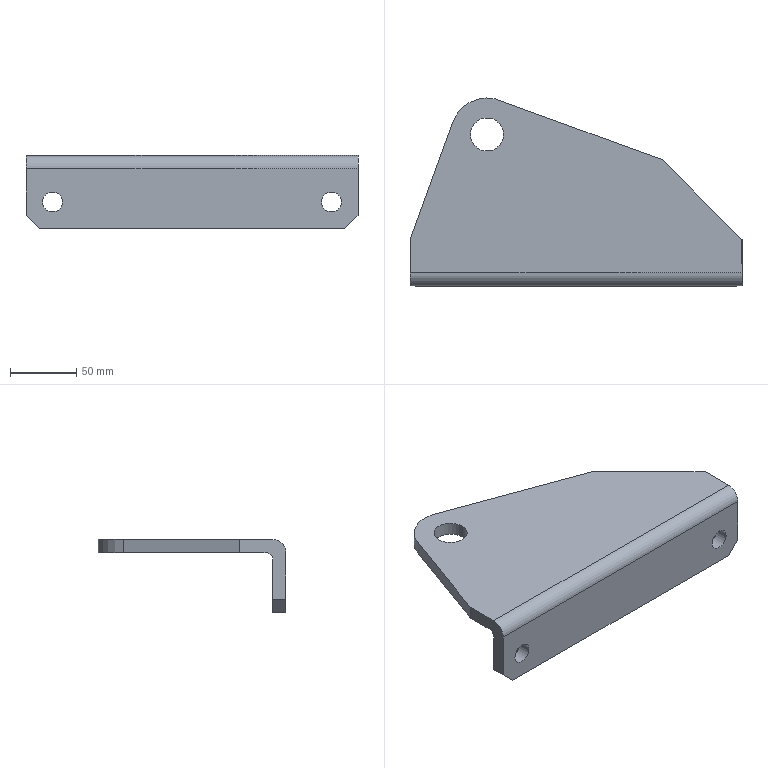Part | SolidWorks | features ICE 4, Fillet 2, Chamfer 1, Extrusion 1 | 1 solid | 21 faces | box 250 x 141.5 x 55 mm | volume 355868 mm3 | plane 12 | cylinder 9 | commonest cylinder face diameters 15 x4 25 x2 10 x1 20 x1 55 x1
STEP:
#1=CARTESIAN_POINT('',(-112.5,-80.5,-25.));
#2=VERTEX_POINT('',#1);
#3=CARTESIAN_POINT('',(-97.5,-80.5,-25.));
#4=VERTEX_POINT('',#3);
#5=CARTESIAN_POINT('',(-105.,-80.5,-25.));
#6=DIRECTION('',(0.,-1.,0.));
#7=DIRECTION('',(0.,0.,-1.));
#8=AXIS2_PLACEMENT_3D('',#5,#6,#7);
#9=CIRCLE('',#8,7.5);
#10=EDGE_CURVE('',#2,#4,#9,.T.);
#11=ORIENTED_EDGE('',*,*,#10,.F.);
#12=CARTESIAN_POINT('',(-112.5,-90.5,-25.));
#13=VERTEX_POINT('',#12);
#14=CARTESIAN_POINT('',(-112.5,-45.5,-25.));
#15=DIRECTION('',(0.,-1.,0.));
#16=VECTOR('',#15,1000.);
#17=LINE('',#14,#16);
#18=EDGE_CURVE('',#2,#13,#17,.T.);
#19=ORIENTED_EDGE('',*,*,#18,.T.);
#20=CARTESIAN_POINT('',(-97.5,-90.5,-25.));
#21=VERTEX_POINT('',#20);
#22=CARTESIAN_POINT('',(-105.,-90.5,-25.));
#23=DIRECTION('',(0.,-1.,0.));
#24=DIRECTION('',(1.,0.,0.));
#25=AXIS2_PLACEMENT_3D('',#22,#23,#24);
#26=CIRCLE('',#25,7.5);
#27=EDGE_CURVE('',#13,#21,#26,.T.);
#28=ORIENTED_EDGE('',*,*,#27,.T.);
#29=CARTESIAN_POINT('',(-97.5,-45.5,-25.));
#30=DIRECTION('',(0.,-1.,0.));
#31=VECTOR('',#30,1000.);
#32=LINE('',#29,#31);
#33=EDGE_CURVE('',#4,#21,#32,.T.);
#34=ORIENTED_EDGE('',*,*,#33,.F.);
#35=EDGE_LOOP('',(#11,#19,#28,#34));
#36=FACE_OUTER_BOUND('',#35,.T.);
#37=CARTESIAN_POINT('',(-105.,-45.5,-25.));
#38=DIRECTION('',(0.,-1.,0.));
#39=DIRECTION('',(1.,0.,0.));
#40=AXIS2_PLACEMENT_3D('',#37,#38,#39);
#41=CYLINDRICAL_SURFACE('',#40,7.5);
#42=ADVANCED_FACE('',(#36),#41,.F.);
#43=CARTESIAN_POINT('',(97.5,-80.5,-25.));
#44=VERTEX_POINT('',#43);
#45=CARTESIAN_POINT('',(112.5,-80.5,-25.));
#46=VERTEX_POINT('',#45);
#47=CARTESIAN_POINT('',(105.,-80.5,-25.));
#48=DIRECTION('',(0.,-1.,0.));
#49=DIRECTION('',(0.,0.,-1.));
#50=AXIS2_PLACEMENT_3D('',#47,#48,#49);
#51=CIRCLE('',#50,7.5);
#52=EDGE_CURVE('',#44,#46,#51,.T.);
#53=ORIENTED_EDGE('',*,*,#52,.F.);
#54=CARTESIAN_POINT('',(97.5,-90.5,-25.));
#55=VERTEX_POINT('',#54);
#56=CARTESIAN_POINT('',(97.5,-45.5,-25.));
#57=DIRECTION('',(0.,-1.,0.));
#58=VECTOR('',#57,1000.);
#59=LINE('',#56,#58);
#60=EDGE_CURVE('',#44,#55,#59,.T.);
#61=ORIENTED_EDGE('',*,*,#60,.T.);
#62=CARTESIAN_POINT('',(112.5,-90.5,-25.));
#63=VERTEX_POINT('',#62);
#64=CARTESIAN_POINT('',(105.,-90.5,-25.));
#65=DIRECTION('',(0.,-1.,0.));
#66=DIRECTION('',(1.,0.,0.));
#67=AXIS2_PLACEMENT_3D('',#64,#65,#66);
#68=CIRCLE('',#67,7.5);
#69=EDGE_CURVE('',#55,#63,#68,.T.);
#70=ORIENTED_EDGE('',*,*,#69,.T.);
#71=CARTESIAN_POINT('',(112.5,-45.5,-25.));
#72=DIRECTION('',(0.,-1.,0.));
#73=VECTOR('',#72,1000.);
#74=LINE('',#71,#73);
#75=EDGE_CURVE('',#46,#63,#74,.T.);
#76=ORIENTED_EDGE('',*,*,#75,.F.);
#77=EDGE_LOOP('',(#53,#61,#70,#76));
#78=FACE_OUTER_BOUND('',#77,.T.);
#79=CARTESIAN_POINT('',(105.,-45.5,-25.));
#80=DIRECTION('',(0.,-1.,0.));
#81=DIRECTION('',(1.,0.,0.));
#82=AXIS2_PLACEMENT_3D('',#79,#80,#81);
#83=CYLINDRICAL_SURFACE('',#82,7.5);
#84=ADVANCED_FACE('',(#78),#83,.F.);
#85=CARTESIAN_POINT('',(-79.5,23.5,0.));
#86=VERTEX_POINT('',#85);
#87=CARTESIAN_POINT('',(-54.5,23.5,0.));
#88=VERTEX_POINT('',#87);
#89=CARTESIAN_POINT('',(-67.,23.5,0.));
#90=DIRECTION('',(0.,0.,1.));
#91=DIRECTION('',(1.,0.,0.));
#92=AXIS2_PLACEMENT_3D('',#89,#90,#91);
#93=CIRCLE('',#92,12.5);
#94=EDGE_CURVE('',#86,#88,#93,.T.);
#95=ORIENTED_EDGE('',*,*,#94,.F.);
#96=CARTESIAN_POINT('',(-79.5,23.5,10.));
#97=VERTEX_POINT('',#96);
#98=CARTESIAN_POINT('',(-79.5,23.5,0.));
#99=DIRECTION('',(0.,0.,1.));
#100=VECTOR('',#99,1000.);
#101=LINE('',#98,#100);
#102=EDGE_CURVE('',#86,#97,#101,.T.);
#103=ORIENTED_EDGE('',*,*,#102,.T.);
#104=CARTESIAN_POINT('',(-54.5,23.5,10.));
#105=VERTEX_POINT('',#104);
#106=CARTESIAN_POINT('',(-67.,23.5,10.));
#107=DIRECTION('',(0.,0.,1.));
#108=DIRECTION('',(1.,0.,0.));
#109=AXIS2_PLACEMENT_3D('',#106,#107,#108);
#110=CIRCLE('',#109,12.5);
#111=EDGE_CURVE('',#97,#105,#110,.T.);
#112=ORIENTED_EDGE('',*,*,#111,.T.);
#113=CARTESIAN_POINT('',(-54.5,23.5,0.));
#114=DIRECTION('',(0.,0.,1.));
#115=VECTOR('',#114,1000.);
#116=LINE('',#113,#115);
#117=EDGE_CURVE('',#88,#105,#116,.T.);
#118=ORIENTED_EDGE('',*,*,#117,.F.);
#119=EDGE_LOOP('',(#95,#103,#112,#118));
#120=FACE_OUTER_BOUND('',#119,.T.);
#121=CARTESIAN_POINT('',(-67.,23.5,0.));
#122=DIRECTION('',(0.,0.,1.));
#123=DIRECTION('',(1.,0.,0.));
#124=AXIS2_PLACEMENT_3D('',#121,#122,#123);
#125=CYLINDRICAL_SURFACE('',#124,12.5);
#126=ADVANCED_FACE('',(#120),#125,.F.);
#127=CARTESIAN_POINT('',(-67.,23.5,0.));
#128=DIRECTION('',(0.,0.,1.));
#129=DIRECTION('',(1.,0.,0.));
#130=AXIS2_PLACEMENT_3D('',#127,#128,#129);
#131=CIRCLE('',#130,12.5);
#132=EDGE_CURVE('',#88,#86,#131,.T.);
#133=ORIENTED_EDGE('',*,*,#132,.T.);
#134=ORIENTED_EDGE('',*,*,#94,.T.);
#135=EDGE_LOOP('',(#133,#134));
#136=FACE_BOUND('',#135,.T.);
#137=CARTESIAN_POINT('',(125.,-55.5,0.));
#138=VERTEX_POINT('',#137);
#139=CARTESIAN_POINT('',(125.,-75.5,0.));
#140=VERTEX_POINT('',#139);
#141=CARTESIAN_POINT('',(125.,90.5,0.));
#142=DIRECTION('',(0.,-1.,0.));
#143=VECTOR('',#142,1000.);
#144=LINE('',#141,#143);
#145=EDGE_CURVE('',#138,#140,#144,.T.);
#146=ORIENTED_EDGE('',*,*,#145,.T.);
#147=CARTESIAN_POINT('',(-125.,-75.5,0.));
#148=VERTEX_POINT('',#147);
#149=CARTESIAN_POINT('',(-125.,-75.5,0.));
#150=DIRECTION('',(-1.,0.,0.));
#151=VECTOR('',#150,1000.);
#152=LINE('',#149,#151);
#153=EDGE_CURVE('',#140,#148,#152,.T.);
#154=ORIENTED_EDGE('',*,*,#153,.T.);
#155=CARTESIAN_POINT('',(-125.,-55.5,0.));
#156=VERTEX_POINT('',#155);
#157=CARTESIAN_POINT('',(-125.,90.5,0.));
#158=DIRECTION('',(0.,-1.,0.));
#159=VECTOR('',#158,1000.);
#160=LINE('',#157,#159);
#161=EDGE_CURVE('',#156,#148,#160,.T.);
#162=ORIENTED_EDGE('',*,*,#161,.F.);
#163=CARTESIAN_POINT('',(-93.16,31.98,0.));
#164=VERTEX_POINT('',#163);
#165=CARTESIAN_POINT('',(-125.,-55.5,0.));
#166=DIRECTION('',(-0.342,-0.9397,0.));
#167=VECTOR('',#166,1000.);
#168=LINE('',#165,#167);
#169=EDGE_CURVE('',#164,#156,#168,.T.);
#170=ORIENTED_EDGE('',*,*,#169,.F.);
#171=CARTESIAN_POINT('',(-54.497,47.993,0.));
#172=VERTEX_POINT('',#171);
#173=CARTESIAN_POINT('',(-67.,23.5,0.));
#174=DIRECTION('',(0.,0.,1.));
#175=DIRECTION('',(1.,0.,0.));
#176=AXIS2_PLACEMENT_3D('',#173,#174,#175);
#177=CIRCLE('',#176,27.5);
#178=EDGE_CURVE('',#172,#164,#177,.T.);
#179=ORIENTED_EDGE('',*,*,#178,.F.);
#180=CARTESIAN_POINT('',(65.,4.5,0.));
#181=VERTEX_POINT('',#180);
#182=CARTESIAN_POINT('',(65.,4.5,0.));
#183=DIRECTION('',(-0.9397,0.342,0.));
#184=VECTOR('',#183,1000.);
#185=LINE('',#182,#184);
#186=EDGE_CURVE('',#181,#172,#185,.T.);
#187=ORIENTED_EDGE('',*,*,#186,.F.);
#188=CARTESIAN_POINT('',(125.,-55.5,0.));
#189=DIRECTION('',(-0.7071,0.7071,0.));
#190=VECTOR('',#189,1000.);
#191=LINE('',#188,#190);
#192=EDGE_CURVE('',#138,#181,#191,.T.);
#193=ORIENTED_EDGE('',*,*,#192,.F.);
#194=EDGE_LOOP('',(#146,#154,#162,#170,#179,#187,#193));
#195=FACE_OUTER_BOUND('',#194,.T.);
#196=CARTESIAN_POINT('',(0.,0.,0.));
#197=DIRECTION('',(0.,0.,1.));
#198=DIRECTION('',(1.,0.,0.));
#199=AXIS2_PLACEMENT_3D('',#196,#197,#198);
#200=PLANE('',#199);
#201=ADVANCED_FACE('',(#136,#195),#200,.F.);
#202=CARTESIAN_POINT('',(125.,-90.5,0.));
#203=VERTEX_POINT('',#202);
#204=CARTESIAN_POINT('',(125.,-90.5,-35.));
#205=VERTEX_POINT('',#204);
#206=CARTESIAN_POINT('',(125.,-90.5,10.));
#207=DIRECTION('',(0.,0.,-1.));
#208=VECTOR('',#207,1000.);
#209=LINE('',#206,#208);
#210=EDGE_CURVE('',#203,#205,#209,.T.);
#211=ORIENTED_EDGE('',*,*,#210,.T.);
#212=CARTESIAN_POINT('',(125.,-80.5,-35.));
#213=VERTEX_POINT('',#212);
#214=CARTESIAN_POINT('',(125.,-80.5,-35.));
#215=DIRECTION('',(0.,1.,0.));
#216=VECTOR('',#215,1000.);
#217=LINE('',#214,#216);
#218=EDGE_CURVE('',#205,#213,#217,.T.);
#219=ORIENTED_EDGE('',*,*,#218,.T.);
#220=CARTESIAN_POINT('',(125.,-80.5,-5.));
#221=VERTEX_POINT('',#220);
#222=CARTESIAN_POINT('',(125.,-80.5,-45.));
#223=DIRECTION('',(0.,0.,1.));
#224=VECTOR('',#223,1000.);
#225=LINE('',#222,#224);
#226=EDGE_CURVE('',#213,#221,#225,.T.);
#227=ORIENTED_EDGE('',*,*,#226,.T.);
#228=CARTESIAN_POINT('',(125.,-75.5,-5.));
#229=DIRECTION('',(-1.,0.,0.));
#230=DIRECTION('',(0.,1.,0.));
#231=AXIS2_PLACEMENT_3D('',#228,#229,#230);
#232=CIRCLE('',#231,5.);
#233=EDGE_CURVE('',#221,#140,#232,.T.);
#234=ORIENTED_EDGE('',*,*,#233,.T.);
#235=ORIENTED_EDGE('',*,*,#145,.F.);
#236=CARTESIAN_POINT('',(125.,-55.5,10.));
#237=VERTEX_POINT('',#236);
#238=CARTESIAN_POINT('',(125.,-55.5,0.));
#239=DIRECTION('',(0.,0.,1.));
#240=VECTOR('',#239,1000.);
#241=LINE('',#238,#240);
#242=EDGE_CURVE('',#138,#237,#241,.T.);
#243=ORIENTED_EDGE('',*,*,#242,.T.);
#244=CARTESIAN_POINT('',(125.,-80.5,10.));
#245=VERTEX_POINT('',#244);
#246=CARTESIAN_POINT('',(125.,90.5,10.));
#247=DIRECTION('',(0.,-1.,0.));
#248=VECTOR('',#247,1000.);
#249=LINE('',#246,#248);
#250=EDGE_CURVE('',#237,#245,#249,.T.);
#251=ORIENTED_EDGE('',*,*,#250,.T.);
#252=CARTESIAN_POINT('',(125.,-80.5,0.));
#253=DIRECTION('',(1.,0.,0.));
#254=DIRECTION('',(0.,1.,0.));
#255=AXIS2_PLACEMENT_3D('',#252,#253,#254);
#256=CIRCLE('',#255,10.);
#257=EDGE_CURVE('',#245,#203,#256,.T.);
#258=ORIENTED_EDGE('',*,*,#257,.T.);
#259=EDGE_LOOP('',(#211,#219,#227,#234,#235,#243,#251,#258));
#260=FACE_OUTER_BOUND('',#259,.T.);
#261=CARTESIAN_POINT('',(125.,90.5,10.));
#262=DIRECTION('',(1.,0.,0.));
#263=DIRECTION('',(0.,1.,0.));
#264=AXIS2_PLACEMENT_3D('',#261,#262,#263);
#265=PLANE('',#264);
#266=ADVANCED_FACE('',(#260),#265,.T.);
#267=CARTESIAN_POINT('',(-125.,-80.5,-35.));
#268=VERTEX_POINT('',#267);
#269=CARTESIAN_POINT('',(-125.,-80.5,-5.));
#270=VERTEX_POINT('',#269);
#271=CARTESIAN_POINT('',(-125.,-80.5,-45.));
#272=DIRECTION('',(0.,0.,1.));
#273=VECTOR('',#272,1000.);
#274=LINE('',#271,#273);
#275=EDGE_CURVE('',#268,#270,#274,.T.);
#276=ORIENTED_EDGE('',*,*,#275,.F.);
#277=CARTESIAN_POINT('',(-125.,-90.5,-35.));
#278=VERTEX_POINT('',#277);
#279=CARTESIAN_POINT('',(-125.,90.5,-35.));
#280=DIRECTION('',(0.,-1.,0.));
#281=VECTOR('',#280,1000.);
#282=LINE('',#279,#281);
#283=EDGE_CURVE('',#268,#278,#282,.T.);
#284=ORIENTED_EDGE('',*,*,#283,.T.);
#285=CARTESIAN_POINT('',(-125.,-90.5,0.));
#286=VERTEX_POINT('',#285);
#287=CARTESIAN_POINT('',(-125.,-90.5,10.));
#288=DIRECTION('',(0.,0.,-1.));
#289=VECTOR('',#288,1000.);
#290=LINE('',#287,#289);
#291=EDGE_CURVE('',#286,#278,#290,.T.);
#292=ORIENTED_EDGE('',*,*,#291,.F.);
#293=CARTESIAN_POINT('',(-125.,-80.5,10.));
#294=VERTEX_POINT('',#293);
#295=CARTESIAN_POINT('',(-125.,-80.5,0.));
#296=DIRECTION('',(-1.,0.,0.));
#297=DIRECTION('',(0.,1.,0.));
#298=AXIS2_PLACEMENT_3D('',#295,#296,#297);
#299=CIRCLE('',#298,10.);
#300=EDGE_CURVE('',#286,#294,#299,.T.);
#301=ORIENTED_EDGE('',*,*,#300,.T.);
#302=CARTESIAN_POINT('',(-125.,-55.5,10.));
#303=VERTEX_POINT('',#302);
#304=CARTESIAN_POINT('',(-125.,90.5,10.));
#305=DIRECTION('',(0.,-1.,0.));
#306=VECTOR('',#305,1000.);
#307=LINE('',#304,#306);
#308=EDGE_CURVE('',#303,#294,#307,.T.);
#309=ORIENTED_EDGE('',*,*,#308,.F.);
#310=CARTESIAN_POINT('',(-125.,-55.5,0.));
#311=DIRECTION('',(0.,0.,1.));
#312=VECTOR('',#311,1000.);
#313=LINE('',#310,#312);
#314=EDGE_CURVE('',#156,#303,#313,.T.);
#315=ORIENTED_EDGE('',*,*,#314,.F.);
#316=ORIENTED_EDGE('',*,*,#161,.T.);
#317=CARTESIAN_POINT('',(-125.,-75.5,-5.));
#318=DIRECTION('',(1.,0.,0.));
#319=DIRECTION('',(0.,1.,0.));
#320=AXIS2_PLACEMENT_3D('',#317,#318,#319);
#321=CIRCLE('',#320,5.);
#322=EDGE_CURVE('',#148,#270,#321,.T.);
#323=ORIENTED_EDGE('',*,*,#322,.T.);
#324=EDGE_LOOP('',(#276,#284,#292,#301,#309,#315,#316,#323));
#325=FACE_OUTER_BOUND('',#324,.T.);
#326=CARTESIAN_POINT('',(-125.,90.5,10.));
#327=DIRECTION('',(1.,0.,0.));
#328=DIRECTION('',(0.,1.,0.));
#329=AXIS2_PLACEMENT_3D('',#326,#327,#328);
#330=PLANE('',#329);
#331=ADVANCED_FACE('',(#325),#330,.F.);
#332=CARTESIAN_POINT('',(-67.,23.5,10.));
#333=DIRECTION('',(0.,0.,1.));
#334=DIRECTION('',(1.,0.,0.));
#335=AXIS2_PLACEMENT_3D('',#332,#333,#334);
#336=CIRCLE('',#335,12.5);
#337=EDGE_CURVE('',#105,#97,#336,.T.);
#338=ORIENTED_EDGE('',*,*,#337,.F.);
#339=ORIENTED_EDGE('',*,*,#111,.F.);
#340=EDGE_LOOP('',(#338,#339));
#341=FACE_BOUND('',#340,.T.);
#342=ORIENTED_EDGE('',*,*,#308,.T.);
#343=CARTESIAN_POINT('',(0.,-80.5,10.));
#344=DIRECTION('',(1.,0.,0.));
#345=VECTOR('',#344,1000.);
#346=LINE('',#343,#345);
#347=EDGE_CURVE('',#294,#245,#346,.T.);
#348=ORIENTED_EDGE('',*,*,#347,.T.);
#349=ORIENTED_EDGE('',*,*,#250,.F.);
#350=CARTESIAN_POINT('',(65.,4.5,10.));
#351=VERTEX_POINT('',#350);
#352=CARTESIAN_POINT('',(125.,-55.5,10.));
#353=DIRECTION('',(-0.7071,0.7071,0.));
#354=VECTOR('',#353,1000.);
#355=LINE('',#352,#354);
#356=EDGE_CURVE('',#237,#351,#355,.T.);
#357=ORIENTED_EDGE('',*,*,#356,.T.);
#358=CARTESIAN_POINT('',(-54.497,47.993,10.));
#359=VERTEX_POINT('',#358);
#360=CARTESIAN_POINT('',(65.,4.5,10.));
#361=DIRECTION('',(-0.9397,0.342,0.));
#362=VECTOR('',#361,1000.);
#363=LINE('',#360,#362);
#364=EDGE_CURVE('',#351,#359,#363,.T.);
#365=ORIENTED_EDGE('',*,*,#364,.T.);
#366=CARTESIAN_POINT('',(-93.16,31.98,10.));
#367=VERTEX_POINT('',#366);
#368=CARTESIAN_POINT('',(-67.,23.5,10.));
#369=DIRECTION('',(0.,0.,1.));
#370=DIRECTION('',(1.,0.,0.));
#371=AXIS2_PLACEMENT_3D('',#368,#369,#370);
#372=CIRCLE('',#371,27.5);
#373=EDGE_CURVE('',#359,#367,#372,.T.);
#374=ORIENTED_EDGE('',*,*,#373,.T.);
#375=CARTESIAN_POINT('',(-125.,-55.5,10.));
#376=DIRECTION('',(-0.342,-0.9397,0.));
#377=VECTOR('',#376,1000.);
#378=LINE('',#375,#377);
#379=EDGE_CURVE('',#367,#303,#378,.T.);
#380=ORIENTED_EDGE('',*,*,#379,.T.);
#381=EDGE_LOOP('',(#342,#348,#349,#357,#365,#374,#380));
#382=FACE_OUTER_BOUND('',#381,.T.);
#383=CARTESIAN_POINT('',(0.,0.,10.));
#384=DIRECTION('',(0.,0.,1.));
#385=DIRECTION('',(1.,0.,0.));
#386=AXIS2_PLACEMENT_3D('',#383,#384,#385);
#387=PLANE('',#386);
#388=ADVANCED_FACE('',(#341,#382),#387,.T.);
#389=CARTESIAN_POINT('',(-105.,-90.5,-25.));
#390=DIRECTION('',(0.,-1.,0.));
#391=DIRECTION('',(1.,0.,0.));
#392=AXIS2_PLACEMENT_3D('',#389,#390,#391);
#393=CIRCLE('',#392,7.5);
#394=EDGE_CURVE('',#21,#13,#393,.T.);
#395=ORIENTED_EDGE('',*,*,#394,.F.);
#396=ORIENTED_EDGE('',*,*,#27,.F.);
#397=EDGE_LOOP('',(#395,#396));
#398=FACE_BOUND('',#397,.T.);
#399=CARTESIAN_POINT('',(105.,-90.5,-25.));
#400=DIRECTION('',(0.,-1.,0.));
#401=DIRECTION('',(1.,0.,0.));
#402=AXIS2_PLACEMENT_3D('',#399,#400,#401);
#403=CIRCLE('',#402,7.5);
#404=EDGE_CURVE('',#63,#55,#403,.T.);
#405=ORIENTED_EDGE('',*,*,#404,.F.);
#406=ORIENTED_EDGE('',*,*,#69,.F.);
#407=EDGE_LOOP('',(#405,#406));
#408=FACE_BOUND('',#407,.T.);
#409=CARTESIAN_POINT('',(115.,-90.5,-45.));
#410=VERTEX_POINT('',#409);
#411=CARTESIAN_POINT('',(-115.,-90.5,-45.));
#412=VERTEX_POINT('',#411);
#413=CARTESIAN_POINT('',(-125.,-90.5,-45.));
#414=DIRECTION('',(-1.,0.,0.));
#415=VECTOR('',#414,1000.);
#416=LINE('',#413,#415);
#417=EDGE_CURVE('',#410,#412,#416,.T.);
#418=ORIENTED_EDGE('',*,*,#417,.F.);
#419=CARTESIAN_POINT('',(147.5,-90.5,-12.5));
#420=DIRECTION('',(0.7071,0.,0.7071));
#421=VECTOR('',#420,1000.);
#422=LINE('',#419,#421);
#423=EDGE_CURVE('',#410,#205,#422,.T.);
#424=ORIENTED_EDGE('',*,*,#423,.T.);
#425=ORIENTED_EDGE('',*,*,#210,.F.);
#426=CARTESIAN_POINT('',(125.,-90.5,0.));
#427=DIRECTION('',(-1.,0.,0.));
#428=VECTOR('',#427,1000.);
#429=LINE('',#426,#428);
#430=EDGE_CURVE('',#203,#286,#429,.T.);
#431=ORIENTED_EDGE('',*,*,#430,.T.);
#432=ORIENTED_EDGE('',*,*,#291,.T.);
#433=CARTESIAN_POINT('',(-22.5,-90.5,-137.5));
#434=DIRECTION('',(0.7071,0.,-0.7071));
#435=VECTOR('',#434,1000.);
#436=LINE('',#433,#435);
#437=EDGE_CURVE('',#278,#412,#436,.T.);
#438=ORIENTED_EDGE('',*,*,#437,.T.);
#439=EDGE_LOOP('',(#418,#424,#425,#431,#432,#438));
#440=FACE_OUTER_BOUND('',#439,.T.);
#441=CARTESIAN_POINT('',(125.,-90.5,10.));
#442=DIRECTION('',(0.,-1.,0.));
#443=DIRECTION('',(1.,0.,0.));
#444=AXIS2_PLACEMENT_3D('',#441,#442,#443);
#445=PLANE('',#444);
#446=ADVANCED_FACE('',(#398,#408,#440),#445,.T.);
#447=ORIENTED_EDGE('',*,*,#379,.F.);
#448=CARTESIAN_POINT('',(-93.16,31.98,0.));
#449=DIRECTION('',(0.,0.,1.));
#450=VECTOR('',#449,1000.);
#451=LINE('',#448,#450);
#452=EDGE_CURVE('',#164,#367,#451,.T.);
#453=ORIENTED_EDGE('',*,*,#452,.F.);
#454=ORIENTED_EDGE('',*,*,#169,.T.);
#455=ORIENTED_EDGE('',*,*,#314,.T.);
#456=EDGE_LOOP('',(#447,#453,#454,#455));
#457=FACE_OUTER_BOUND('',#456,.T.);
#458=CARTESIAN_POINT('',(-125.,-55.5,0.));
#459=DIRECTION('',(-0.9397,0.342,0.));
#460=DIRECTION('',(-0.342,-0.9397,0.));
#461=AXIS2_PLACEMENT_3D('',#458,#459,#460);
#462=PLANE('',#461);
#463=ADVANCED_FACE('',(#457),#462,.T.);
#464=ORIENTED_EDGE('',*,*,#373,.F.);
#465=CARTESIAN_POINT('',(-54.497,47.993,0.));
#466=DIRECTION('',(0.,0.,1.));
#467=VECTOR('',#466,1000.);
#468=LINE('',#465,#467);
#469=EDGE_CURVE('',#172,#359,#468,.T.);
#470=ORIENTED_EDGE('',*,*,#469,.F.);
#471=ORIENTED_EDGE('',*,*,#178,.T.);
#472=ORIENTED_EDGE('',*,*,#452,.T.);
#473=EDGE_LOOP('',(#464,#470,#471,#472));
#474=FACE_OUTER_BOUND('',#473,.T.);
#475=CARTESIAN_POINT('',(-67.,23.5,0.));
#476=DIRECTION('',(0.,0.,1.));
#477=DIRECTION('',(1.,0.,0.));
#478=AXIS2_PLACEMENT_3D('',#475,#476,#477);
#479=CYLINDRICAL_SURFACE('',#478,27.5);
#480=ADVANCED_FACE('',(#474),#479,.T.);
#481=ORIENTED_EDGE('',*,*,#364,.F.);
#482=CARTESIAN_POINT('',(65.,4.5,0.));
#483=DIRECTION('',(0.,0.,1.));
#484=VECTOR('',#483,1000.);
#485=LINE('',#482,#484);
#486=EDGE_CURVE('',#181,#351,#485,.T.);
#487=ORIENTED_EDGE('',*,*,#486,.F.);
#488=ORIENTED_EDGE('',*,*,#186,.T.);
#489=ORIENTED_EDGE('',*,*,#469,.T.);
#490=EDGE_LOOP('',(#481,#487,#488,#489));
#491=FACE_OUTER_BOUND('',#490,.T.);
#492=CARTESIAN_POINT('',(65.,4.5,0.));
#493=DIRECTION('',(0.342,0.9397,0.));
#494=DIRECTION('',(-0.9397,0.342,0.));
#495=AXIS2_PLACEMENT_3D('',#492,#493,#494);
#496=PLANE('',#495);
#497=ADVANCED_FACE('',(#491),#496,.T.);
#498=ORIENTED_EDGE('',*,*,#356,.F.);
#499=ORIENTED_EDGE('',*,*,#242,.F.);
#500=ORIENTED_EDGE('',*,*,#192,.T.);
#501=ORIENTED_EDGE('',*,*,#486,.T.);
#502=EDGE_LOOP('',(#498,#499,#500,#501));
#503=FACE_OUTER_BOUND('',#502,.T.);
#504=CARTESIAN_POINT('',(125.,-55.5,0.));
#505=DIRECTION('',(0.7071,0.7071,0.));
#506=DIRECTION('',(-0.7071,0.7071,0.));
#507=AXIS2_PLACEMENT_3D('',#504,#505,#506);
#508=PLANE('',#507);
#509=ADVANCED_FACE('',(#503),#508,.T.);
#510=ORIENTED_EDGE('',*,*,#102,.F.);
#511=ORIENTED_EDGE('',*,*,#132,.F.);
#512=ORIENTED_EDGE('',*,*,#117,.T.);
#513=ORIENTED_EDGE('',*,*,#337,.T.);
#514=EDGE_LOOP('',(#510,#511,#512,#513));
#515=FACE_OUTER_BOUND('',#514,.T.);
#516=CARTESIAN_POINT('',(-67.,23.5,0.));
#517=DIRECTION('',(0.,0.,1.));
#518=DIRECTION('',(1.,0.,0.));
#519=AXIS2_PLACEMENT_3D('',#516,#517,#518);
#520=CYLINDRICAL_SURFACE('',#519,12.5);
#521=ADVANCED_FACE('',(#515),#520,.F.);
#522=CARTESIAN_POINT('',(-105.,-80.5,-25.));
#523=DIRECTION('',(0.,-1.,0.));
#524=DIRECTION('',(0.,0.,-1.));
#525=AXIS2_PLACEMENT_3D('',#522,#523,#524);
#526=CIRCLE('',#525,7.5);
#527=EDGE_CURVE('',#4,#2,#526,.T.);
#528=ORIENTED_EDGE('',*,*,#527,.T.);
#529=ORIENTED_EDGE('',*,*,#10,.T.);
#530=EDGE_LOOP('',(#528,#529));
#531=FACE_BOUND('',#530,.T.);
#532=CARTESIAN_POINT('',(105.,-80.5,-25.));
#533=DIRECTION('',(0.,-1.,0.));
#534=DIRECTION('',(0.,0.,-1.));
#535=AXIS2_PLACEMENT_3D('',#532,#533,#534);
#536=CIRCLE('',#535,7.5);
#537=EDGE_CURVE('',#46,#44,#536,.T.);
#538=ORIENTED_EDGE('',*,*,#537,.T.);
#539=ORIENTED_EDGE('',*,*,#52,.T.);
#540=EDGE_LOOP('',(#538,#539));
#541=FACE_BOUND('',#540,.T.);
#542=ORIENTED_EDGE('',*,*,#226,.F.);
#543=CARTESIAN_POINT('',(115.,-80.5,-45.));
#544=VERTEX_POINT('',#543);
#545=CARTESIAN_POINT('',(115.,-80.5,-45.));
#546=DIRECTION('',(-0.7071,0.,-0.7071));
#547=VECTOR('',#546,1000.);
#548=LINE('',#545,#547);
#549=EDGE_CURVE('',#213,#544,#548,.T.);
#550=ORIENTED_EDGE('',*,*,#549,.T.);
#551=CARTESIAN_POINT('',(-115.,-80.5,-45.));
#552=VERTEX_POINT('',#551);
#553=CARTESIAN_POINT('',(125.,-80.5,-45.));
#554=DIRECTION('',(1.,0.,0.));
#555=VECTOR('',#554,1000.);
#556=LINE('',#553,#555);
#557=EDGE_CURVE('',#552,#544,#556,.T.);
#558=ORIENTED_EDGE('',*,*,#557,.F.);
#559=CARTESIAN_POINT('',(-115.,-80.5,-45.));
#560=DIRECTION('',(-0.7071,0.,0.7071));
#561=VECTOR('',#560,1000.);
#562=LINE('',#559,#561);
#563=EDGE_CURVE('',#552,#268,#562,.T.);
#564=ORIENTED_EDGE('',*,*,#563,.T.);
#565=ORIENTED_EDGE('',*,*,#275,.T.);
#566=CARTESIAN_POINT('',(125.,-80.5,-5.));
#567=DIRECTION('',(1.,0.,0.));
#568=VECTOR('',#567,1000.);
#569=LINE('',#566,#568);
#570=EDGE_CURVE('',#270,#221,#569,.T.);
#571=ORIENTED_EDGE('',*,*,#570,.T.);
#572=EDGE_LOOP('',(#542,#550,#558,#564,#565,#571));
#573=FACE_OUTER_BOUND('',#572,.T.);
#574=CARTESIAN_POINT('',(125.,-80.5,-45.));
#575=DIRECTION('',(0.,-1.,0.));
#576=DIRECTION('',(0.,0.,-1.));
#577=AXIS2_PLACEMENT_3D('',#574,#575,#576);
#578=PLANE('',#577);
#579=ADVANCED_FACE('',(#531,#541,#573),#578,.F.);
#580=ORIENTED_EDGE('',*,*,#557,.T.);
#581=CARTESIAN_POINT('',(115.,-90.5,-45.));
#582=DIRECTION('',(0.,-1.,0.));
#583=VECTOR('',#582,1000.);
#584=LINE('',#581,#583);
#585=EDGE_CURVE('',#544,#410,#584,.T.);
#586=ORIENTED_EDGE('',*,*,#585,.T.);
#587=ORIENTED_EDGE('',*,*,#417,.T.);
#588=CARTESIAN_POINT('',(-115.,0.,-45.));
#589=DIRECTION('',(0.,1.,0.));
#590=VECTOR('',#589,1000.);
#591=LINE('',#588,#590);
#592=EDGE_CURVE('',#412,#552,#591,.T.);
#593=ORIENTED_EDGE('',*,*,#592,.T.);
#594=EDGE_LOOP('',(#580,#586,#587,#593));
#595=FACE_OUTER_BOUND('',#594,.T.);
#596=CARTESIAN_POINT('',(0.,0.,-45.));
#597=DIRECTION('',(0.,0.,1.));
#598=DIRECTION('',(1.,0.,0.));
#599=AXIS2_PLACEMENT_3D('',#596,#597,#598);
#600=PLANE('',#599);
#601=ADVANCED_FACE('',(#595),#600,.F.);
#602=ORIENTED_EDGE('',*,*,#257,.F.);
#603=ORIENTED_EDGE('',*,*,#347,.F.);
#604=ORIENTED_EDGE('',*,*,#300,.F.);
#605=ORIENTED_EDGE('',*,*,#430,.F.);
#606=EDGE_LOOP('',(#602,#603,#604,#605));
#607=FACE_OUTER_BOUND('',#606,.T.);
#608=CARTESIAN_POINT('',(125.,-80.5,0.));
#609=DIRECTION('',(-1.,0.,0.));
#610=DIRECTION('',(0.,-1.,0.));
#611=AXIS2_PLACEMENT_3D('',#608,#609,#610);
#612=CYLINDRICAL_SURFACE('',#611,10.);
#613=ADVANCED_FACE('',(#607),#612,.T.);
#614=ORIENTED_EDGE('',*,*,#322,.F.);
#615=ORIENTED_EDGE('',*,*,#153,.F.);
#616=ORIENTED_EDGE('',*,*,#233,.F.);
#617=ORIENTED_EDGE('',*,*,#570,.F.);
#618=EDGE_LOOP('',(#614,#615,#616,#617));
#619=FACE_OUTER_BOUND('',#618,.T.);
#620=CARTESIAN_POINT('',(125.,-75.5,-5.));
#621=DIRECTION('',(-1.,0.,0.));
#622=DIRECTION('',(0.,0.,1.));
#623=AXIS2_PLACEMENT_3D('',#620,#621,#622);
#624=CYLINDRICAL_SURFACE('',#623,5.);
#625=ADVANCED_FACE('',(#619),#624,.F.);
#626=ORIENTED_EDGE('',*,*,#60,.F.);
#627=ORIENTED_EDGE('',*,*,#537,.F.);
#628=ORIENTED_EDGE('',*,*,#75,.T.);
#629=ORIENTED_EDGE('',*,*,#404,.T.);
#630=EDGE_LOOP('',(#626,#627,#628,#629));
#631=FACE_OUTER_BOUND('',#630,.T.);
#632=CARTESIAN_POINT('',(105.,-45.5,-25.));
#633=DIRECTION('',(0.,-1.,0.));
#634=DIRECTION('',(1.,0.,0.));
#635=AXIS2_PLACEMENT_3D('',#632,#633,#634);
#636=CYLINDRICAL_SURFACE('',#635,7.5);
#637=ADVANCED_FACE('',(#631),#636,.F.);
#638=ORIENTED_EDGE('',*,*,#18,.F.);
#639=ORIENTED_EDGE('',*,*,#527,.F.);
#640=ORIENTED_EDGE('',*,*,#33,.T.);
#641=ORIENTED_EDGE('',*,*,#394,.T.);
#642=EDGE_LOOP('',(#638,#639,#640,#641));
#643=FACE_OUTER_BOUND('',#642,.T.);
#644=CARTESIAN_POINT('',(-105.,-45.5,-25.));
#645=DIRECTION('',(0.,-1.,0.));
#646=DIRECTION('',(1.,0.,0.));
#647=AXIS2_PLACEMENT_3D('',#644,#645,#646);
#648=CYLINDRICAL_SURFACE('',#647,7.5);
#649=ADVANCED_FACE('',(#643),#648,.F.);
#650=ORIENTED_EDGE('',*,*,#549,.F.);
#651=ORIENTED_EDGE('',*,*,#218,.F.);
#652=ORIENTED_EDGE('',*,*,#423,.F.);
#653=ORIENTED_EDGE('',*,*,#585,.F.);
#654=EDGE_LOOP('',(#650,#651,#652,#653));
#655=FACE_OUTER_BOUND('',#654,.T.);
#656=CARTESIAN_POINT('',(115.,0.,-45.));
#657=DIRECTION('',(0.7071,0.,-0.7071));
#658=DIRECTION('',(0.,1.,0.));
#659=AXIS2_PLACEMENT_3D('',#656,#657,#658);
#660=PLANE('',#659);
#661=ADVANCED_FACE('',(#655),#660,.T.);
#662=ORIENTED_EDGE('',*,*,#437,.F.);
#663=ORIENTED_EDGE('',*,*,#283,.F.);
#664=ORIENTED_EDGE('',*,*,#563,.F.);
#665=ORIENTED_EDGE('',*,*,#592,.F.);
#666=EDGE_LOOP('',(#662,#663,#664,#665));
#667=FACE_OUTER_BOUND('',#666,.T.);
#668=CARTESIAN_POINT('',(-115.,0.,-45.));
#669=DIRECTION('',(0.7071,0.,0.7071));
#670=DIRECTION('',(0.,1.,0.));
#671=AXIS2_PLACEMENT_3D('',#668,#669,#670);
#672=PLANE('',#671);
#673=ADVANCED_FACE('',(#667),#672,.F.);
#674=CLOSED_SHELL('',(#42,#84,#126,#201,#266,#331,#388,#446,#463,#480,#497,#509,#521,#579,#601,#613,#625,#637,#649,#661,#673));
#675=MANIFOLD_SOLID_BREP('',#674);
#676=CARTESIAN_POINT('',(0.,0.,0.));
#677=DIRECTION('',(0.,0.,1.));
#678=DIRECTION('',(1.,0.,0.));
#679=AXIS2_PLACEMENT_3D('',#676,#677,#678);
#680=(LENGTH_UNIT()NAMED_UNIT(*)SI_UNIT(.MILLI.,.METRE.));
#681=UNCERTAINTY_MEASURE_WITH_UNIT(LENGTH_MEASURE(0.00001),#680,'','');
#682=(NAMED_UNIT(*)PLANE_ANGLE_UNIT()SI_UNIT($,.RADIAN.));
#683=(NAMED_UNIT(*)SI_UNIT($,.STERADIAN.)SOLID_ANGLE_UNIT());
#684=(GEOMETRIC_REPRESENTATION_CONTEXT(3)GLOBAL_UNCERTAINTY_ASSIGNED_CONTEXT((#681))GLOBAL_UNIT_ASSIGNED_CONTEXT((#680,#682,#683))REPRESENTATION_CONTEXT('',''));
#685=ADVANCED_BREP_SHAPE_REPRESENTATION('',(#675,#679),#684);